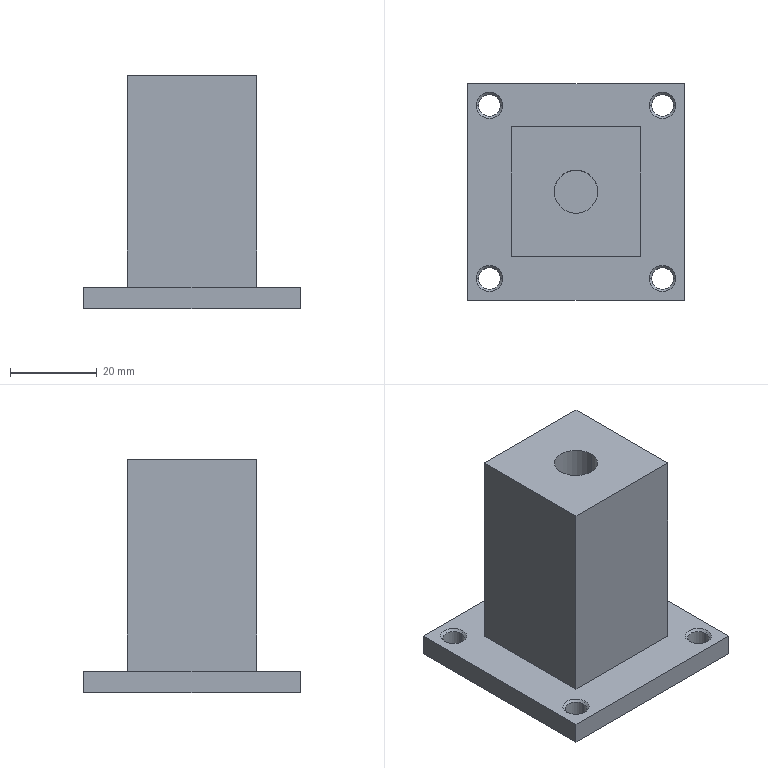Part | SolidWorks | features Cut 1, Extrusion 1, HoleWzd 1, ICE 1 | 1 solid | 30 faces | box 50 x 50 x 54 mm | volume 53135 mm3 | plane 12 | cylinder 10 | cone 8 | commonest cylinder face diameters 5 x8 10 x2
STEP:
#1=CARTESIAN_POINT('',(-55.,0.,15.));
#2=VERTEX_POINT('',#1);
#3=CARTESIAN_POINT('',(-45.,0.,15.));
#4=VERTEX_POINT('',#3);
#5=CARTESIAN_POINT('',(-50.,0.,15.));
#6=DIRECTION('',(0.,0.,1.));
#7=DIRECTION('',(1.,0.,0.));
#8=AXIS2_PLACEMENT_3D('',#5,#6,#7);
#9=CIRCLE('',#8,5.);
#10=EDGE_CURVE('',#2,#4,#9,.T.);
#11=ORIENTED_EDGE('',*,*,#10,.F.);
#12=CARTESIAN_POINT('',(-55.,0.,54.));
#13=VERTEX_POINT('',#12);
#14=CARTESIAN_POINT('',(-55.,0.,15.));
#15=DIRECTION('',(0.,0.,1.));
#16=VECTOR('',#15,1000.);
#17=LINE('',#14,#16);
#18=EDGE_CURVE('',#2,#13,#17,.T.);
#19=ORIENTED_EDGE('',*,*,#18,.T.);
#20=CARTESIAN_POINT('',(-45.,0.,54.));
#21=VERTEX_POINT('',#20);
#22=CARTESIAN_POINT('',(-50.,0.,54.));
#23=DIRECTION('',(0.,0.,1.));
#24=DIRECTION('',(1.,0.,0.));
#25=AXIS2_PLACEMENT_3D('',#22,#23,#24);
#26=CIRCLE('',#25,5.);
#27=EDGE_CURVE('',#13,#21,#26,.T.);
#28=ORIENTED_EDGE('',*,*,#27,.T.);
#29=CARTESIAN_POINT('',(-45.,0.,15.));
#30=DIRECTION('',(0.,0.,1.));
#31=VECTOR('',#30,1000.);
#32=LINE('',#29,#31);
#33=EDGE_CURVE('',#4,#21,#32,.T.);
#34=ORIENTED_EDGE('',*,*,#33,.F.);
#35=EDGE_LOOP('',(#11,#19,#28,#34));
#36=FACE_OUTER_BOUND('',#35,.T.);
#37=CARTESIAN_POINT('',(-50.,0.,15.));
#38=DIRECTION('',(0.,0.,1.));
#39=DIRECTION('',(1.,0.,0.));
#40=AXIS2_PLACEMENT_3D('',#37,#38,#39);
#41=CYLINDRICAL_SURFACE('',#40,5.);
#42=ADVANCED_FACE('',(#36),#41,.F.);
#43=CARTESIAN_POINT('',(-32.5,20.,4.475));
#44=VERTEX_POINT('',#43);
#45=CARTESIAN_POINT('',(-27.5,20.,4.475));
#46=VERTEX_POINT('',#45);
#47=CARTESIAN_POINT('',(-30.,20.,4.475));
#48=DIRECTION('',(0.,0.,1.));
#49=DIRECTION('',(1.,0.,0.));
#50=AXIS2_PLACEMENT_3D('',#47,#48,#49);
#51=CIRCLE('',#50,2.5);
#52=EDGE_CURVE('',#44,#46,#51,.T.);
#53=ORIENTED_EDGE('',*,*,#52,.F.);
#54=CARTESIAN_POINT('',(-33.025,20.,5.));
#55=VERTEX_POINT('',#54);
#56=CARTESIAN_POINT('',(-33.025,20.,5.));
#57=DIRECTION('',(-0.7071,0.,0.7071));
#58=VECTOR('',#57,1000.);
#59=LINE('',#56,#58);
#60=EDGE_CURVE('',#44,#55,#59,.T.);
#61=ORIENTED_EDGE('',*,*,#60,.T.);
#62=CARTESIAN_POINT('',(-26.975,20.,5.));
#63=VERTEX_POINT('',#62);
#64=CARTESIAN_POINT('',(-30.,20.,5.));
#65=DIRECTION('',(0.,0.,1.));
#66=DIRECTION('',(1.,0.,0.));
#67=AXIS2_PLACEMENT_3D('',#64,#65,#66);
#68=CIRCLE('',#67,3.025);
#69=EDGE_CURVE('',#55,#63,#68,.T.);
#70=ORIENTED_EDGE('',*,*,#69,.T.);
#71=CARTESIAN_POINT('',(-26.975,20.,5.));
#72=DIRECTION('',(0.7071,0.,0.7071));
#73=VECTOR('',#72,1000.);
#74=LINE('',#71,#73);
#75=EDGE_CURVE('',#46,#63,#74,.T.);
#76=ORIENTED_EDGE('',*,*,#75,.F.);
#77=EDGE_LOOP('',(#53,#61,#70,#76));
#78=FACE_OUTER_BOUND('',#77,.T.);
#79=CARTESIAN_POINT('',(-30.,20.,5.));
#80=DIRECTION('',(0.,0.,1.));
#81=DIRECTION('',(1.,0.,0.));
#82=AXIS2_PLACEMENT_3D('',#79,#80,#81);
#83=CONICAL_SURFACE('',#82,3.025,0.7854);
#84=ADVANCED_FACE('',(#78),#83,.F.);
#85=CARTESIAN_POINT('',(-27.5,20.,0.));
#86=VERTEX_POINT('',#85);
#87=CARTESIAN_POINT('',(-32.5,20.,0.));
#88=VERTEX_POINT('',#87);
#89=CARTESIAN_POINT('',(-30.,20.,0.));
#90=DIRECTION('',(0.,0.,-1.));
#91=DIRECTION('',(-1.,0.,0.));
#92=AXIS2_PLACEMENT_3D('',#89,#90,#91);
#93=CIRCLE('',#92,2.5);
#94=EDGE_CURVE('',#86,#88,#93,.T.);
#95=ORIENTED_EDGE('',*,*,#94,.T.);
#96=CARTESIAN_POINT('',(-32.5,20.,5.));
#97=DIRECTION('',(0.,0.,1.));
#98=VECTOR('',#97,1000.);
#99=LINE('',#96,#98);
#100=EDGE_CURVE('',#88,#44,#99,.T.);
#101=ORIENTED_EDGE('',*,*,#100,.T.);
#102=ORIENTED_EDGE('',*,*,#52,.T.);
#103=CARTESIAN_POINT('',(-27.5,20.,5.));
#104=DIRECTION('',(0.,0.,1.));
#105=VECTOR('',#104,1000.);
#106=LINE('',#103,#105);
#107=EDGE_CURVE('',#86,#46,#106,.T.);
#108=ORIENTED_EDGE('',*,*,#107,.F.);
#109=EDGE_LOOP('',(#95,#101,#102,#108));
#110=FACE_OUTER_BOUND('',#109,.T.);
#111=CARTESIAN_POINT('',(-30.,20.,5.));
#112=DIRECTION('',(0.,0.,1.));
#113=DIRECTION('',(1.,0.,0.));
#114=AXIS2_PLACEMENT_3D('',#111,#112,#113);
#115=CYLINDRICAL_SURFACE('',#114,2.5);
#116=ADVANCED_FACE('',(#110),#115,.F.);
#117=CARTESIAN_POINT('',(-72.5,20.,4.475));
#118=VERTEX_POINT('',#117);
#119=CARTESIAN_POINT('',(-67.5,20.,4.475));
#120=VERTEX_POINT('',#119);
#121=CARTESIAN_POINT('',(-70.,20.,4.475));
#122=DIRECTION('',(0.,0.,1.));
#123=DIRECTION('',(1.,0.,0.));
#124=AXIS2_PLACEMENT_3D('',#121,#122,#123);
#125=CIRCLE('',#124,2.5);
#126=EDGE_CURVE('',#118,#120,#125,.T.);
#127=ORIENTED_EDGE('',*,*,#126,.F.);
#128=CARTESIAN_POINT('',(-73.025,20.,5.));
#129=VERTEX_POINT('',#128);
#130=CARTESIAN_POINT('',(-73.025,20.,5.));
#131=DIRECTION('',(-0.7071,0.,0.7071));
#132=VECTOR('',#131,1000.);
#133=LINE('',#130,#132);
#134=EDGE_CURVE('',#118,#129,#133,.T.);
#135=ORIENTED_EDGE('',*,*,#134,.T.);
#136=CARTESIAN_POINT('',(-66.975,20.,5.));
#137=VERTEX_POINT('',#136);
#138=CARTESIAN_POINT('',(-70.,20.,5.));
#139=DIRECTION('',(0.,0.,1.));
#140=DIRECTION('',(1.,0.,0.));
#141=AXIS2_PLACEMENT_3D('',#138,#139,#140);
#142=CIRCLE('',#141,3.025);
#143=EDGE_CURVE('',#129,#137,#142,.T.);
#144=ORIENTED_EDGE('',*,*,#143,.T.);
#145=CARTESIAN_POINT('',(-66.975,20.,5.));
#146=DIRECTION('',(0.7071,0.,0.7071));
#147=VECTOR('',#146,1000.);
#148=LINE('',#145,#147);
#149=EDGE_CURVE('',#120,#137,#148,.T.);
#150=ORIENTED_EDGE('',*,*,#149,.F.);
#151=EDGE_LOOP('',(#127,#135,#144,#150));
#152=FACE_OUTER_BOUND('',#151,.T.);
#153=CARTESIAN_POINT('',(-70.,20.,5.));
#154=DIRECTION('',(0.,0.,1.));
#155=DIRECTION('',(1.,0.,0.));
#156=AXIS2_PLACEMENT_3D('',#153,#154,#155);
#157=CONICAL_SURFACE('',#156,3.025,0.7854);
#158=ADVANCED_FACE('',(#152),#157,.F.);
#159=CARTESIAN_POINT('',(-67.5,20.,0.));
#160=VERTEX_POINT('',#159);
#161=CARTESIAN_POINT('',(-72.5,20.,0.));
#162=VERTEX_POINT('',#161);
#163=CARTESIAN_POINT('',(-70.,20.,0.));
#164=DIRECTION('',(0.,0.,-1.));
#165=DIRECTION('',(-1.,0.,0.));
#166=AXIS2_PLACEMENT_3D('',#163,#164,#165);
#167=CIRCLE('',#166,2.5);
#168=EDGE_CURVE('',#160,#162,#167,.T.);
#169=ORIENTED_EDGE('',*,*,#168,.T.);
#170=CARTESIAN_POINT('',(-72.5,20.,5.));
#171=DIRECTION('',(0.,0.,1.));
#172=VECTOR('',#171,1000.);
#173=LINE('',#170,#172);
#174=EDGE_CURVE('',#162,#118,#173,.T.);
#175=ORIENTED_EDGE('',*,*,#174,.T.);
#176=ORIENTED_EDGE('',*,*,#126,.T.);
#177=CARTESIAN_POINT('',(-67.5,20.,5.));
#178=DIRECTION('',(0.,0.,1.));
#179=VECTOR('',#178,1000.);
#180=LINE('',#177,#179);
#181=EDGE_CURVE('',#160,#120,#180,.T.);
#182=ORIENTED_EDGE('',*,*,#181,.F.);
#183=EDGE_LOOP('',(#169,#175,#176,#182));
#184=FACE_OUTER_BOUND('',#183,.T.);
#185=CARTESIAN_POINT('',(-70.,20.,5.));
#186=DIRECTION('',(0.,0.,1.));
#187=DIRECTION('',(1.,0.,0.));
#188=AXIS2_PLACEMENT_3D('',#185,#186,#187);
#189=CYLINDRICAL_SURFACE('',#188,2.5);
#190=ADVANCED_FACE('',(#184),#189,.F.);
#191=CARTESIAN_POINT('',(-72.5,-20.,4.475));
#192=VERTEX_POINT('',#191);
#193=CARTESIAN_POINT('',(-67.5,-20.,4.475));
#194=VERTEX_POINT('',#193);
#195=CARTESIAN_POINT('',(-70.,-20.,4.475));
#196=DIRECTION('',(0.,0.,1.));
#197=DIRECTION('',(1.,0.,0.));
#198=AXIS2_PLACEMENT_3D('',#195,#196,#197);
#199=CIRCLE('',#198,2.5);
#200=EDGE_CURVE('',#192,#194,#199,.T.);
#201=ORIENTED_EDGE('',*,*,#200,.F.);
#202=CARTESIAN_POINT('',(-73.025,-20.,5.));
#203=VERTEX_POINT('',#202);
#204=CARTESIAN_POINT('',(-73.025,-20.,5.));
#205=DIRECTION('',(-0.7071,0.,0.7071));
#206=VECTOR('',#205,1000.);
#207=LINE('',#204,#206);
#208=EDGE_CURVE('',#192,#203,#207,.T.);
#209=ORIENTED_EDGE('',*,*,#208,.T.);
#210=CARTESIAN_POINT('',(-66.975,-20.,5.));
#211=VERTEX_POINT('',#210);
#212=CARTESIAN_POINT('',(-70.,-20.,5.));
#213=DIRECTION('',(0.,0.,1.));
#214=DIRECTION('',(1.,0.,0.));
#215=AXIS2_PLACEMENT_3D('',#212,#213,#214);
#216=CIRCLE('',#215,3.025);
#217=EDGE_CURVE('',#203,#211,#216,.T.);
#218=ORIENTED_EDGE('',*,*,#217,.T.);
#219=CARTESIAN_POINT('',(-66.975,-20.,5.));
#220=DIRECTION('',(0.7071,0.,0.7071));
#221=VECTOR('',#220,1000.);
#222=LINE('',#219,#221);
#223=EDGE_CURVE('',#194,#211,#222,.T.);
#224=ORIENTED_EDGE('',*,*,#223,.F.);
#225=EDGE_LOOP('',(#201,#209,#218,#224));
#226=FACE_OUTER_BOUND('',#225,.T.);
#227=CARTESIAN_POINT('',(-70.,-20.,5.));
#228=DIRECTION('',(0.,0.,1.));
#229=DIRECTION('',(1.,0.,0.));
#230=AXIS2_PLACEMENT_3D('',#227,#228,#229);
#231=CONICAL_SURFACE('',#230,3.025,0.7854);
#232=ADVANCED_FACE('',(#226),#231,.F.);
#233=CARTESIAN_POINT('',(-67.5,-20.,0.));
#234=VERTEX_POINT('',#233);
#235=CARTESIAN_POINT('',(-72.5,-20.,0.));
#236=VERTEX_POINT('',#235);
#237=CARTESIAN_POINT('',(-70.,-20.,0.));
#238=DIRECTION('',(0.,0.,-1.));
#239=DIRECTION('',(-1.,0.,0.));
#240=AXIS2_PLACEMENT_3D('',#237,#238,#239);
#241=CIRCLE('',#240,2.5);
#242=EDGE_CURVE('',#234,#236,#241,.T.);
#243=ORIENTED_EDGE('',*,*,#242,.T.);
#244=CARTESIAN_POINT('',(-72.5,-20.,5.));
#245=DIRECTION('',(0.,0.,1.));
#246=VECTOR('',#245,1000.);
#247=LINE('',#244,#246);
#248=EDGE_CURVE('',#236,#192,#247,.T.);
#249=ORIENTED_EDGE('',*,*,#248,.T.);
#250=ORIENTED_EDGE('',*,*,#200,.T.);
#251=CARTESIAN_POINT('',(-67.5,-20.,5.));
#252=DIRECTION('',(0.,0.,1.));
#253=VECTOR('',#252,1000.);
#254=LINE('',#251,#253);
#255=EDGE_CURVE('',#234,#194,#254,.T.);
#256=ORIENTED_EDGE('',*,*,#255,.F.);
#257=EDGE_LOOP('',(#243,#249,#250,#256));
#258=FACE_OUTER_BOUND('',#257,.T.);
#259=CARTESIAN_POINT('',(-70.,-20.,5.));
#260=DIRECTION('',(0.,0.,1.));
#261=DIRECTION('',(1.,0.,0.));
#262=AXIS2_PLACEMENT_3D('',#259,#260,#261);
#263=CYLINDRICAL_SURFACE('',#262,2.5);
#264=ADVANCED_FACE('',(#258),#263,.F.);
#265=CARTESIAN_POINT('',(-32.5,-20.,4.475));
#266=VERTEX_POINT('',#265);
#267=CARTESIAN_POINT('',(-27.5,-20.,4.475));
#268=VERTEX_POINT('',#267);
#269=CARTESIAN_POINT('',(-30.,-20.,4.475));
#270=DIRECTION('',(0.,0.,1.));
#271=DIRECTION('',(1.,0.,0.));
#272=AXIS2_PLACEMENT_3D('',#269,#270,#271);
#273=CIRCLE('',#272,2.5);
#274=EDGE_CURVE('',#266,#268,#273,.T.);
#275=ORIENTED_EDGE('',*,*,#274,.F.);
#276=CARTESIAN_POINT('',(-33.025,-20.,5.));
#277=VERTEX_POINT('',#276);
#278=CARTESIAN_POINT('',(-33.025,-20.,5.));
#279=DIRECTION('',(-0.7071,0.,0.7071));
#280=VECTOR('',#279,1000.);
#281=LINE('',#278,#280);
#282=EDGE_CURVE('',#266,#277,#281,.T.);
#283=ORIENTED_EDGE('',*,*,#282,.T.);
#284=CARTESIAN_POINT('',(-26.975,-20.,5.));
#285=VERTEX_POINT('',#284);
#286=CARTESIAN_POINT('',(-30.,-20.,5.));
#287=DIRECTION('',(0.,0.,1.));
#288=DIRECTION('',(1.,0.,0.));
#289=AXIS2_PLACEMENT_3D('',#286,#287,#288);
#290=CIRCLE('',#289,3.025);
#291=EDGE_CURVE('',#277,#285,#290,.T.);
#292=ORIENTED_EDGE('',*,*,#291,.T.);
#293=CARTESIAN_POINT('',(-26.975,-20.,5.));
#294=DIRECTION('',(0.7071,0.,0.7071));
#295=VECTOR('',#294,1000.);
#296=LINE('',#293,#295);
#297=EDGE_CURVE('',#268,#285,#296,.T.);
#298=ORIENTED_EDGE('',*,*,#297,.F.);
#299=EDGE_LOOP('',(#275,#283,#292,#298));
#300=FACE_OUTER_BOUND('',#299,.T.);
#301=CARTESIAN_POINT('',(-30.,-20.,5.));
#302=DIRECTION('',(0.,0.,1.));
#303=DIRECTION('',(1.,0.,0.));
#304=AXIS2_PLACEMENT_3D('',#301,#302,#303);
#305=CONICAL_SURFACE('',#304,3.025,0.7854);
#306=ADVANCED_FACE('',(#300),#305,.F.);
#307=CARTESIAN_POINT('',(-27.5,-20.,0.));
#308=VERTEX_POINT('',#307);
#309=CARTESIAN_POINT('',(-32.5,-20.,0.));
#310=VERTEX_POINT('',#309);
#311=CARTESIAN_POINT('',(-30.,-20.,0.));
#312=DIRECTION('',(0.,0.,-1.));
#313=DIRECTION('',(-1.,0.,0.));
#314=AXIS2_PLACEMENT_3D('',#311,#312,#313);
#315=CIRCLE('',#314,2.5);
#316=EDGE_CURVE('',#308,#310,#315,.T.);
#317=ORIENTED_EDGE('',*,*,#316,.T.);
#318=CARTESIAN_POINT('',(-32.5,-20.,5.));
#319=DIRECTION('',(0.,0.,1.));
#320=VECTOR('',#319,1000.);
#321=LINE('',#318,#320);
#322=EDGE_CURVE('',#310,#266,#321,.T.);
#323=ORIENTED_EDGE('',*,*,#322,.T.);
#324=ORIENTED_EDGE('',*,*,#274,.T.);
#325=CARTESIAN_POINT('',(-27.5,-20.,5.));
#326=DIRECTION('',(0.,0.,1.));
#327=VECTOR('',#326,1000.);
#328=LINE('',#325,#327);
#329=EDGE_CURVE('',#308,#268,#328,.T.);
#330=ORIENTED_EDGE('',*,*,#329,.F.);
#331=EDGE_LOOP('',(#317,#323,#324,#330));
#332=FACE_OUTER_BOUND('',#331,.T.);
#333=CARTESIAN_POINT('',(-30.,-20.,5.));
#334=DIRECTION('',(0.,0.,1.));
#335=DIRECTION('',(1.,0.,0.));
#336=AXIS2_PLACEMENT_3D('',#333,#334,#335);
#337=CYLINDRICAL_SURFACE('',#336,2.5);
#338=ADVANCED_FACE('',(#332),#337,.F.);
#339=CARTESIAN_POINT('',(-65.,15.,54.));
#340=VERTEX_POINT('',#339);
#341=CARTESIAN_POINT('',(-65.,15.,5.));
#342=VERTEX_POINT('',#341);
#343=CARTESIAN_POINT('',(-65.,15.,54.));
#344=DIRECTION('',(0.,0.,-1.));
#345=VECTOR('',#344,1000.);
#346=LINE('',#343,#345);
#347=EDGE_CURVE('',#340,#342,#346,.T.);
#348=ORIENTED_EDGE('',*,*,#347,.T.);
#349=CARTESIAN_POINT('',(-65.,-15.,5.));
#350=VERTEX_POINT('',#349);
#351=CARTESIAN_POINT('',(-65.,15.,5.));
#352=DIRECTION('',(0.,-1.,0.));
#353=VECTOR('',#352,1000.);
#354=LINE('',#351,#353);
#355=EDGE_CURVE('',#342,#350,#354,.T.);
#356=ORIENTED_EDGE('',*,*,#355,.T.);
#357=CARTESIAN_POINT('',(-65.,-15.,54.));
#358=VERTEX_POINT('',#357);
#359=CARTESIAN_POINT('',(-65.,-15.,54.));
#360=DIRECTION('',(0.,0.,-1.));
#361=VECTOR('',#360,1000.);
#362=LINE('',#359,#361);
#363=EDGE_CURVE('',#358,#350,#362,.T.);
#364=ORIENTED_EDGE('',*,*,#363,.F.);
#365=CARTESIAN_POINT('',(-65.,15.,54.));
#366=DIRECTION('',(0.,-1.,0.));
#367=VECTOR('',#366,1000.);
#368=LINE('',#365,#367);
#369=EDGE_CURVE('',#340,#358,#368,.T.);
#370=ORIENTED_EDGE('',*,*,#369,.F.);
#371=EDGE_LOOP('',(#348,#356,#364,#370));
#372=FACE_OUTER_BOUND('',#371,.T.);
#373=CARTESIAN_POINT('',(-65.,15.,54.));
#374=DIRECTION('',(1.,0.,0.));
#375=DIRECTION('',(0.,0.,-1.));
#376=AXIS2_PLACEMENT_3D('',#373,#374,#375);
#377=PLANE('',#376);
#378=ADVANCED_FACE('',(#372),#377,.F.);
#379=ORIENTED_EDGE('',*,*,#363,.T.);
#380=CARTESIAN_POINT('',(-35.,-15.,5.));
#381=VERTEX_POINT('',#380);
#382=CARTESIAN_POINT('',(-35.,-15.,5.));
#383=DIRECTION('',(1.,0.,0.));
#384=VECTOR('',#383,1000.);
#385=LINE('',#382,#384);
#386=EDGE_CURVE('',#350,#381,#385,.T.);
#387=ORIENTED_EDGE('',*,*,#386,.T.);
#388=CARTESIAN_POINT('',(-35.,-15.,54.));
#389=VERTEX_POINT('',#388);
#390=CARTESIAN_POINT('',(-35.,-15.,54.));
#391=DIRECTION('',(0.,0.,-1.));
#392=VECTOR('',#391,1000.);
#393=LINE('',#390,#392);
#394=EDGE_CURVE('',#389,#381,#393,.T.);
#395=ORIENTED_EDGE('',*,*,#394,.F.);
#396=CARTESIAN_POINT('',(-35.,-15.,54.));
#397=DIRECTION('',(1.,0.,0.));
#398=VECTOR('',#397,1000.);
#399=LINE('',#396,#398);
#400=EDGE_CURVE('',#358,#389,#399,.T.);
#401=ORIENTED_EDGE('',*,*,#400,.F.);
#402=EDGE_LOOP('',(#379,#387,#395,#401));
#403=FACE_OUTER_BOUND('',#402,.T.);
#404=CARTESIAN_POINT('',(-35.,-15.,54.));
#405=DIRECTION('',(0.,1.,0.));
#406=DIRECTION('',(-1.,0.,0.));
#407=AXIS2_PLACEMENT_3D('',#404,#405,#406);
#408=PLANE('',#407);
#409=ADVANCED_FACE('',(#403),#408,.F.);
#410=ORIENTED_EDGE('',*,*,#394,.T.);
#411=CARTESIAN_POINT('',(-35.,15.,5.));
#412=VERTEX_POINT('',#411);
#413=CARTESIAN_POINT('',(-35.,15.,5.));
#414=DIRECTION('',(0.,1.,0.));
#415=VECTOR('',#414,1000.);
#416=LINE('',#413,#415);
#417=EDGE_CURVE('',#381,#412,#416,.T.);
#418=ORIENTED_EDGE('',*,*,#417,.T.);
#419=CARTESIAN_POINT('',(-35.,15.,54.));
#420=VERTEX_POINT('',#419);
#421=CARTESIAN_POINT('',(-35.,15.,54.));
#422=DIRECTION('',(0.,0.,-1.));
#423=VECTOR('',#422,1000.);
#424=LINE('',#421,#423);
#425=EDGE_CURVE('',#420,#412,#424,.T.);
#426=ORIENTED_EDGE('',*,*,#425,.F.);
#427=CARTESIAN_POINT('',(-35.,15.,54.));
#428=DIRECTION('',(0.,1.,0.));
#429=VECTOR('',#428,1000.);
#430=LINE('',#427,#429);
#431=EDGE_CURVE('',#389,#420,#430,.T.);
#432=ORIENTED_EDGE('',*,*,#431,.F.);
#433=EDGE_LOOP('',(#410,#418,#426,#432));
#434=FACE_OUTER_BOUND('',#433,.T.);
#435=CARTESIAN_POINT('',(-35.,15.,54.));
#436=DIRECTION('',(-1.,0.,0.));
#437=DIRECTION('',(0.,-1.,0.));
#438=AXIS2_PLACEMENT_3D('',#435,#436,#437);
#439=PLANE('',#438);
#440=ADVANCED_FACE('',(#434),#439,.F.);
#441=ORIENTED_EDGE('',*,*,#425,.T.);
#442=CARTESIAN_POINT('',(-35.,15.,5.));
#443=DIRECTION('',(-1.,0.,0.));
#444=VECTOR('',#443,1000.);
#445=LINE('',#442,#444);
#446=EDGE_CURVE('',#412,#342,#445,.T.);
#447=ORIENTED_EDGE('',*,*,#446,.T.);
#448=ORIENTED_EDGE('',*,*,#347,.F.);
#449=CARTESIAN_POINT('',(-35.,15.,54.));
#450=DIRECTION('',(-1.,0.,0.));
#451=VECTOR('',#450,1000.);
#452=LINE('',#449,#451);
#453=EDGE_CURVE('',#420,#340,#452,.T.);
#454=ORIENTED_EDGE('',*,*,#453,.F.);
#455=EDGE_LOOP('',(#441,#447,#448,#454));
#456=FACE_OUTER_BOUND('',#455,.T.);
#457=CARTESIAN_POINT('',(-35.,15.,54.));
#458=DIRECTION('',(0.,-1.,0.));
#459=DIRECTION('',(1.,0.,0.));
#460=AXIS2_PLACEMENT_3D('',#457,#458,#459);
#461=PLANE('',#460);
#462=ADVANCED_FACE('',(#456),#461,.F.);
#463=CARTESIAN_POINT('',(-50.,0.,54.));
#464=DIRECTION('',(0.,0.,1.));
#465=DIRECTION('',(1.,0.,0.));
#466=AXIS2_PLACEMENT_3D('',#463,#464,#465);
#467=CIRCLE('',#466,5.);
#468=EDGE_CURVE('',#21,#13,#467,.T.);
#469=ORIENTED_EDGE('',*,*,#468,.F.);
#470=ORIENTED_EDGE('',*,*,#27,.F.);
#471=EDGE_LOOP('',(#469,#470));
#472=FACE_BOUND('',#471,.T.);
#473=ORIENTED_EDGE('',*,*,#369,.T.);
#474=ORIENTED_EDGE('',*,*,#400,.T.);
#475=ORIENTED_EDGE('',*,*,#431,.T.);
#476=ORIENTED_EDGE('',*,*,#453,.T.);
#477=EDGE_LOOP('',(#473,#474,#475,#476));
#478=FACE_OUTER_BOUND('',#477,.T.);
#479=CARTESIAN_POINT('',(0.,0.,54.));
#480=DIRECTION('',(0.,0.,-1.));
#481=DIRECTION('',(-1.,0.,0.));
#482=AXIS2_PLACEMENT_3D('',#479,#480,#481);
#483=PLANE('',#482);
#484=ADVANCED_FACE('',(#472,#478),#483,.F.);
#485=CARTESIAN_POINT('',(-30.,20.,5.));
#486=DIRECTION('',(0.,0.,1.));
#487=DIRECTION('',(1.,0.,0.));
#488=AXIS2_PLACEMENT_3D('',#485,#486,#487);
#489=CIRCLE('',#488,3.025);
#490=EDGE_CURVE('',#63,#55,#489,.T.);
#491=ORIENTED_EDGE('',*,*,#490,.F.);
#492=ORIENTED_EDGE('',*,*,#69,.F.);
#493=EDGE_LOOP('',(#491,#492));
#494=FACE_BOUND('',#493,.T.);
#495=CARTESIAN_POINT('',(-70.,20.,5.));
#496=DIRECTION('',(0.,0.,1.));
#497=DIRECTION('',(1.,0.,0.));
#498=AXIS2_PLACEMENT_3D('',#495,#496,#497);
#499=CIRCLE('',#498,3.025);
#500=EDGE_CURVE('',#137,#129,#499,.T.);
#501=ORIENTED_EDGE('',*,*,#500,.F.);
#502=ORIENTED_EDGE('',*,*,#143,.F.);
#503=EDGE_LOOP('',(#501,#502));
#504=FACE_BOUND('',#503,.T.);
#505=CARTESIAN_POINT('',(-70.,-20.,5.));
#506=DIRECTION('',(0.,0.,1.));
#507=DIRECTION('',(1.,0.,0.));
#508=AXIS2_PLACEMENT_3D('',#505,#506,#507);
#509=CIRCLE('',#508,3.025);
#510=EDGE_CURVE('',#211,#203,#509,.T.);
#511=ORIENTED_EDGE('',*,*,#510,.F.);
#512=ORIENTED_EDGE('',*,*,#217,.F.);
#513=EDGE_LOOP('',(#511,#512));
#514=FACE_BOUND('',#513,.T.);
#515=CARTESIAN_POINT('',(-30.,-20.,5.));
#516=DIRECTION('',(0.,0.,1.));
#517=DIRECTION('',(1.,0.,0.));
#518=AXIS2_PLACEMENT_3D('',#515,#516,#517);
#519=CIRCLE('',#518,3.025);
#520=EDGE_CURVE('',#285,#277,#519,.T.);
#521=ORIENTED_EDGE('',*,*,#520,.F.);
#522=ORIENTED_EDGE('',*,*,#291,.F.);
#523=EDGE_LOOP('',(#521,#522));
#524=FACE_BOUND('',#523,.T.);
#525=CARTESIAN_POINT('',(-25.,25.,5.));
#526=VERTEX_POINT('',#525);
#527=CARTESIAN_POINT('',(-75.,25.,5.));
#528=VERTEX_POINT('',#527);
#529=CARTESIAN_POINT('',(-25.,25.,5.));
#530=DIRECTION('',(-1.,0.,0.));
#531=VECTOR('',#530,1000.);
#532=LINE('',#529,#531);
#533=EDGE_CURVE('',#526,#528,#532,.T.);
#534=ORIENTED_EDGE('',*,*,#533,.T.);
#535=CARTESIAN_POINT('',(-75.,-25.,5.));
#536=VERTEX_POINT('',#535);
#537=CARTESIAN_POINT('',(-75.,25.,5.));
#538=DIRECTION('',(0.,-1.,0.));
#539=VECTOR('',#538,1000.);
#540=LINE('',#537,#539);
#541=EDGE_CURVE('',#528,#536,#540,.T.);
#542=ORIENTED_EDGE('',*,*,#541,.T.);
#543=CARTESIAN_POINT('',(-25.,-25.,5.));
#544=VERTEX_POINT('',#543);
#545=CARTESIAN_POINT('',(-75.,-25.,5.));
#546=DIRECTION('',(1.,0.,0.));
#547=VECTOR('',#546,1000.);
#548=LINE('',#545,#547);
#549=EDGE_CURVE('',#536,#544,#548,.T.);
#550=ORIENTED_EDGE('',*,*,#549,.T.);
#551=CARTESIAN_POINT('',(-25.,-25.,5.));
#552=DIRECTION('',(0.,1.,0.));
#553=VECTOR('',#552,1000.);
#554=LINE('',#551,#553);
#555=EDGE_CURVE('',#544,#526,#554,.T.);
#556=ORIENTED_EDGE('',*,*,#555,.T.);
#557=EDGE_LOOP('',(#534,#542,#550,#556));
#558=FACE_OUTER_BOUND('',#557,.T.);
#559=ORIENTED_EDGE('',*,*,#355,.F.);
#560=ORIENTED_EDGE('',*,*,#446,.F.);
#561=ORIENTED_EDGE('',*,*,#417,.F.);
#562=ORIENTED_EDGE('',*,*,#386,.F.);
#563=EDGE_LOOP('',(#559,#560,#561,#562));
#564=FACE_BOUND('',#563,.T.);
#565=CARTESIAN_POINT('',(0.,0.,5.));
#566=DIRECTION('',(0.,0.,1.));
#567=DIRECTION('',(1.,0.,0.));
#568=AXIS2_PLACEMENT_3D('',#565,#566,#567);
#569=PLANE('',#568);
#570=ADVANCED_FACE('',(#494,#504,#514,#524,#558,#564),#569,.T.);
#571=CARTESIAN_POINT('',(-25.,25.,0.));
#572=VERTEX_POINT('',#571);
#573=CARTESIAN_POINT('',(-75.,25.,0.));
#574=VERTEX_POINT('',#573);
#575=CARTESIAN_POINT('',(-25.,25.,0.));
#576=DIRECTION('',(-1.,0.,0.));
#577=VECTOR('',#576,1000.);
#578=LINE('',#575,#577);
#579=EDGE_CURVE('',#572,#574,#578,.T.);
#580=ORIENTED_EDGE('',*,*,#579,.T.);
#581=CARTESIAN_POINT('',(-75.,25.,5.));
#582=DIRECTION('',(0.,0.,-1.));
#583=VECTOR('',#582,1000.);
#584=LINE('',#581,#583);
#585=EDGE_CURVE('',#528,#574,#584,.T.);
#586=ORIENTED_EDGE('',*,*,#585,.F.);
#587=ORIENTED_EDGE('',*,*,#533,.F.);
#588=CARTESIAN_POINT('',(-25.,25.,5.));
#589=DIRECTION('',(0.,0.,-1.));
#590=VECTOR('',#589,1000.);
#591=LINE('',#588,#590);
#592=EDGE_CURVE('',#526,#572,#591,.T.);
#593=ORIENTED_EDGE('',*,*,#592,.T.);
#594=EDGE_LOOP('',(#580,#586,#587,#593));
#595=FACE_OUTER_BOUND('',#594,.T.);
#596=CARTESIAN_POINT('',(-25.,25.,5.));
#597=DIRECTION('',(0.,-1.,0.));
#598=DIRECTION('',(1.,0.,0.));
#599=AXIS2_PLACEMENT_3D('',#596,#597,#598);
#600=PLANE('',#599);
#601=ADVANCED_FACE('',(#595),#600,.F.);
#602=CARTESIAN_POINT('',(-75.,-25.,0.));
#603=VERTEX_POINT('',#602);
#604=CARTESIAN_POINT('',(-75.,25.,0.));
#605=DIRECTION('',(0.,-1.,0.));
#606=VECTOR('',#605,1000.);
#607=LINE('',#604,#606);
#608=EDGE_CURVE('',#574,#603,#607,.T.);
#609=ORIENTED_EDGE('',*,*,#608,.T.);
#610=CARTESIAN_POINT('',(-75.,-25.,5.));
#611=DIRECTION('',(0.,0.,-1.));
#612=VECTOR('',#611,1000.);
#613=LINE('',#610,#612);
#614=EDGE_CURVE('',#536,#603,#613,.T.);
#615=ORIENTED_EDGE('',*,*,#614,.F.);
#616=ORIENTED_EDGE('',*,*,#541,.F.);
#617=ORIENTED_EDGE('',*,*,#585,.T.);
#618=EDGE_LOOP('',(#609,#615,#616,#617));
#619=FACE_OUTER_BOUND('',#618,.T.);
#620=CARTESIAN_POINT('',(-75.,25.,5.));
#621=DIRECTION('',(1.,0.,0.));
#622=DIRECTION('',(0.,0.,-1.));
#623=AXIS2_PLACEMENT_3D('',#620,#621,#622);
#624=PLANE('',#623);
#625=ADVANCED_FACE('',(#619),#624,.F.);
#626=CARTESIAN_POINT('',(-25.,-25.,0.));
#627=VERTEX_POINT('',#626);
#628=CARTESIAN_POINT('',(-75.,-25.,0.));
#629=DIRECTION('',(1.,0.,0.));
#630=VECTOR('',#629,1000.);
#631=LINE('',#628,#630);
#632=EDGE_CURVE('',#603,#627,#631,.T.);
#633=ORIENTED_EDGE('',*,*,#632,.T.);
#634=CARTESIAN_POINT('',(-25.,-25.,5.));
#635=DIRECTION('',(0.,0.,-1.));
#636=VECTOR('',#635,1000.);
#637=LINE('',#634,#636);
#638=EDGE_CURVE('',#544,#627,#637,.T.);
#639=ORIENTED_EDGE('',*,*,#638,.F.);
#640=ORIENTED_EDGE('',*,*,#549,.F.);
#641=ORIENTED_EDGE('',*,*,#614,.T.);
#642=EDGE_LOOP('',(#633,#639,#640,#641));
#643=FACE_OUTER_BOUND('',#642,.T.);
#644=CARTESIAN_POINT('',(-75.,-25.,5.));
#645=DIRECTION('',(0.,1.,0.));
#646=DIRECTION('',(-1.,0.,0.));
#647=AXIS2_PLACEMENT_3D('',#644,#645,#646);
#648=PLANE('',#647);
#649=ADVANCED_FACE('',(#643),#648,.F.);
#650=CARTESIAN_POINT('',(-25.,-25.,0.));
#651=DIRECTION('',(0.,1.,0.));
#652=VECTOR('',#651,1000.);
#653=LINE('',#650,#652);
#654=EDGE_CURVE('',#627,#572,#653,.T.);
#655=ORIENTED_EDGE('',*,*,#654,.T.);
#656=ORIENTED_EDGE('',*,*,#592,.F.);
#657=ORIENTED_EDGE('',*,*,#555,.F.);
#658=ORIENTED_EDGE('',*,*,#638,.T.);
#659=EDGE_LOOP('',(#655,#656,#657,#658));
#660=FACE_OUTER_BOUND('',#659,.T.);
#661=CARTESIAN_POINT('',(-25.,-25.,5.));
#662=DIRECTION('',(-1.,0.,0.));
#663=DIRECTION('',(0.,-1.,0.));
#664=AXIS2_PLACEMENT_3D('',#661,#662,#663);
#665=PLANE('',#664);
#666=ADVANCED_FACE('',(#660),#665,.F.);
#667=ORIENTED_EDGE('',*,*,#94,.F.);
#668=CARTESIAN_POINT('',(-30.,20.,0.));
#669=DIRECTION('',(0.,0.,-1.));
#670=DIRECTION('',(-1.,0.,0.));
#671=AXIS2_PLACEMENT_3D('',#668,#669,#670);
#672=CIRCLE('',#671,2.5);
#673=EDGE_CURVE('',#88,#86,#672,.T.);
#674=ORIENTED_EDGE('',*,*,#673,.F.);
#675=EDGE_LOOP('',(#667,#674));
#676=FACE_BOUND('',#675,.T.);
#677=ORIENTED_EDGE('',*,*,#168,.F.);
#678=CARTESIAN_POINT('',(-70.,20.,0.));
#679=DIRECTION('',(0.,0.,-1.));
#680=DIRECTION('',(-1.,0.,0.));
#681=AXIS2_PLACEMENT_3D('',#678,#679,#680);
#682=CIRCLE('',#681,2.5);
#683=EDGE_CURVE('',#162,#160,#682,.T.);
#684=ORIENTED_EDGE('',*,*,#683,.F.);
#685=EDGE_LOOP('',(#677,#684));
#686=FACE_BOUND('',#685,.T.);
#687=ORIENTED_EDGE('',*,*,#242,.F.);
#688=CARTESIAN_POINT('',(-70.,-20.,0.));
#689=DIRECTION('',(0.,0.,-1.));
#690=DIRECTION('',(-1.,0.,0.));
#691=AXIS2_PLACEMENT_3D('',#688,#689,#690);
#692=CIRCLE('',#691,2.5);
#693=EDGE_CURVE('',#236,#234,#692,.T.);
#694=ORIENTED_EDGE('',*,*,#693,.F.);
#695=EDGE_LOOP('',(#687,#694));
#696=FACE_BOUND('',#695,.T.);
#697=ORIENTED_EDGE('',*,*,#316,.F.);
#698=CARTESIAN_POINT('',(-30.,-20.,0.));
#699=DIRECTION('',(0.,0.,-1.));
#700=DIRECTION('',(-1.,0.,0.));
#701=AXIS2_PLACEMENT_3D('',#698,#699,#700);
#702=CIRCLE('',#701,2.5);
#703=EDGE_CURVE('',#310,#308,#702,.T.);
#704=ORIENTED_EDGE('',*,*,#703,.F.);
#705=EDGE_LOOP('',(#697,#704));
#706=FACE_BOUND('',#705,.T.);
#707=ORIENTED_EDGE('',*,*,#579,.F.);
#708=ORIENTED_EDGE('',*,*,#654,.F.);
#709=ORIENTED_EDGE('',*,*,#632,.F.);
#710=ORIENTED_EDGE('',*,*,#608,.F.);
#711=EDGE_LOOP('',(#707,#708,#709,#710));
#712=FACE_OUTER_BOUND('',#711,.T.);
#713=CARTESIAN_POINT('',(0.,0.,0.));
#714=DIRECTION('',(0.,0.,-1.));
#715=DIRECTION('',(-1.,0.,0.));
#716=AXIS2_PLACEMENT_3D('',#713,#714,#715);
#717=PLANE('',#716);
#718=ADVANCED_FACE('',(#676,#686,#696,#706,#712),#717,.T.);
#719=ORIENTED_EDGE('',*,*,#322,.F.);
#720=ORIENTED_EDGE('',*,*,#703,.T.);
#721=ORIENTED_EDGE('',*,*,#329,.T.);
#722=CARTESIAN_POINT('',(-30.,-20.,4.475));
#723=DIRECTION('',(0.,0.,1.));
#724=DIRECTION('',(1.,0.,0.));
#725=AXIS2_PLACEMENT_3D('',#722,#723,#724);
#726=CIRCLE('',#725,2.5);
#727=EDGE_CURVE('',#268,#266,#726,.T.);
#728=ORIENTED_EDGE('',*,*,#727,.T.);
#729=EDGE_LOOP('',(#719,#720,#721,#728));
#730=FACE_OUTER_BOUND('',#729,.T.);
#731=CARTESIAN_POINT('',(-30.,-20.,5.));
#732=DIRECTION('',(0.,0.,1.));
#733=DIRECTION('',(1.,0.,0.));
#734=AXIS2_PLACEMENT_3D('',#731,#732,#733);
#735=CYLINDRICAL_SURFACE('',#734,2.5);
#736=ADVANCED_FACE('',(#730),#735,.F.);
#737=ORIENTED_EDGE('',*,*,#282,.F.);
#738=ORIENTED_EDGE('',*,*,#727,.F.);
#739=ORIENTED_EDGE('',*,*,#297,.T.);
#740=ORIENTED_EDGE('',*,*,#520,.T.);
#741=EDGE_LOOP('',(#737,#738,#739,#740));
#742=FACE_OUTER_BOUND('',#741,.T.);
#743=CARTESIAN_POINT('',(-30.,-20.,5.));
#744=DIRECTION('',(0.,0.,1.));
#745=DIRECTION('',(1.,0.,0.));
#746=AXIS2_PLACEMENT_3D('',#743,#744,#745);
#747=CONICAL_SURFACE('',#746,3.025,0.7854);
#748=ADVANCED_FACE('',(#742),#747,.F.);
#749=ORIENTED_EDGE('',*,*,#248,.F.);
#750=ORIENTED_EDGE('',*,*,#693,.T.);
#751=ORIENTED_EDGE('',*,*,#255,.T.);
#752=CARTESIAN_POINT('',(-70.,-20.,4.475));
#753=DIRECTION('',(0.,0.,1.));
#754=DIRECTION('',(1.,0.,0.));
#755=AXIS2_PLACEMENT_3D('',#752,#753,#754);
#756=CIRCLE('',#755,2.5);
#757=EDGE_CURVE('',#194,#192,#756,.T.);
#758=ORIENTED_EDGE('',*,*,#757,.T.);
#759=EDGE_LOOP('',(#749,#750,#751,#758));
#760=FACE_OUTER_BOUND('',#759,.T.);
#761=CARTESIAN_POINT('',(-70.,-20.,5.));
#762=DIRECTION('',(0.,0.,1.));
#763=DIRECTION('',(1.,0.,0.));
#764=AXIS2_PLACEMENT_3D('',#761,#762,#763);
#765=CYLINDRICAL_SURFACE('',#764,2.5);
#766=ADVANCED_FACE('',(#760),#765,.F.);
#767=ORIENTED_EDGE('',*,*,#208,.F.);
#768=ORIENTED_EDGE('',*,*,#757,.F.);
#769=ORIENTED_EDGE('',*,*,#223,.T.);
#770=ORIENTED_EDGE('',*,*,#510,.T.);
#771=EDGE_LOOP('',(#767,#768,#769,#770));
#772=FACE_OUTER_BOUND('',#771,.T.);
#773=CARTESIAN_POINT('',(-70.,-20.,5.));
#774=DIRECTION('',(0.,0.,1.));
#775=DIRECTION('',(1.,0.,0.));
#776=AXIS2_PLACEMENT_3D('',#773,#774,#775);
#777=CONICAL_SURFACE('',#776,3.025,0.7854);
#778=ADVANCED_FACE('',(#772),#777,.F.);
#779=ORIENTED_EDGE('',*,*,#174,.F.);
#780=ORIENTED_EDGE('',*,*,#683,.T.);
#781=ORIENTED_EDGE('',*,*,#181,.T.);
#782=CARTESIAN_POINT('',(-70.,20.,4.475));
#783=DIRECTION('',(0.,0.,1.));
#784=DIRECTION('',(1.,0.,0.));
#785=AXIS2_PLACEMENT_3D('',#782,#783,#784);
#786=CIRCLE('',#785,2.5);
#787=EDGE_CURVE('',#120,#118,#786,.T.);
#788=ORIENTED_EDGE('',*,*,#787,.T.);
#789=EDGE_LOOP('',(#779,#780,#781,#788));
#790=FACE_OUTER_BOUND('',#789,.T.);
#791=CARTESIAN_POINT('',(-70.,20.,5.));
#792=DIRECTION('',(0.,0.,1.));
#793=DIRECTION('',(1.,0.,0.));
#794=AXIS2_PLACEMENT_3D('',#791,#792,#793);
#795=CYLINDRICAL_SURFACE('',#794,2.5);
#796=ADVANCED_FACE('',(#790),#795,.F.);
#797=ORIENTED_EDGE('',*,*,#134,.F.);
#798=ORIENTED_EDGE('',*,*,#787,.F.);
#799=ORIENTED_EDGE('',*,*,#149,.T.);
#800=ORIENTED_EDGE('',*,*,#500,.T.);
#801=EDGE_LOOP('',(#797,#798,#799,#800));
#802=FACE_OUTER_BOUND('',#801,.T.);
#803=CARTESIAN_POINT('',(-70.,20.,5.));
#804=DIRECTION('',(0.,0.,1.));
#805=DIRECTION('',(1.,0.,0.));
#806=AXIS2_PLACEMENT_3D('',#803,#804,#805);
#807=CONICAL_SURFACE('',#806,3.025,0.7854);
#808=ADVANCED_FACE('',(#802),#807,.F.);
#809=ORIENTED_EDGE('',*,*,#100,.F.);
#810=ORIENTED_EDGE('',*,*,#673,.T.);
#811=ORIENTED_EDGE('',*,*,#107,.T.);
#812=CARTESIAN_POINT('',(-30.,20.,4.475));
#813=DIRECTION('',(0.,0.,1.));
#814=DIRECTION('',(1.,0.,0.));
#815=AXIS2_PLACEMENT_3D('',#812,#813,#814);
#816=CIRCLE('',#815,2.5);
#817=EDGE_CURVE('',#46,#44,#816,.T.);
#818=ORIENTED_EDGE('',*,*,#817,.T.);
#819=EDGE_LOOP('',(#809,#810,#811,#818));
#820=FACE_OUTER_BOUND('',#819,.T.);
#821=CARTESIAN_POINT('',(-30.,20.,5.));
#822=DIRECTION('',(0.,0.,1.));
#823=DIRECTION('',(1.,0.,0.));
#824=AXIS2_PLACEMENT_3D('',#821,#822,#823);
#825=CYLINDRICAL_SURFACE('',#824,2.5);
#826=ADVANCED_FACE('',(#820),#825,.F.);
#827=ORIENTED_EDGE('',*,*,#60,.F.);
#828=ORIENTED_EDGE('',*,*,#817,.F.);
#829=ORIENTED_EDGE('',*,*,#75,.T.);
#830=ORIENTED_EDGE('',*,*,#490,.T.);
#831=EDGE_LOOP('',(#827,#828,#829,#830));
#832=FACE_OUTER_BOUND('',#831,.T.);
#833=CARTESIAN_POINT('',(-30.,20.,5.));
#834=DIRECTION('',(0.,0.,1.));
#835=DIRECTION('',(1.,0.,0.));
#836=AXIS2_PLACEMENT_3D('',#833,#834,#835);
#837=CONICAL_SURFACE('',#836,3.025,0.7854);
#838=ADVANCED_FACE('',(#832),#837,.F.);
#839=ORIENTED_EDGE('',*,*,#18,.F.);
#840=CARTESIAN_POINT('',(-50.,0.,15.));
#841=DIRECTION('',(0.,0.,1.));
#842=DIRECTION('',(1.,0.,0.));
#843=AXIS2_PLACEMENT_3D('',#840,#841,#842);
#844=CIRCLE('',#843,5.);
#845=EDGE_CURVE('',#4,#2,#844,.T.);
#846=ORIENTED_EDGE('',*,*,#845,.F.);
#847=ORIENTED_EDGE('',*,*,#33,.T.);
#848=ORIENTED_EDGE('',*,*,#468,.T.);
#849=EDGE_LOOP('',(#839,#846,#847,#848));
#850=FACE_OUTER_BOUND('',#849,.T.);
#851=CARTESIAN_POINT('',(-50.,0.,15.));
#852=DIRECTION('',(0.,0.,1.));
#853=DIRECTION('',(1.,0.,0.));
#854=AXIS2_PLACEMENT_3D('',#851,#852,#853);
#855=CYLINDRICAL_SURFACE('',#854,5.);
#856=ADVANCED_FACE('',(#850),#855,.F.);
#857=ORIENTED_EDGE('',*,*,#845,.T.);
#858=ORIENTED_EDGE('',*,*,#10,.T.);
#859=EDGE_LOOP('',(#857,#858));
#860=FACE_OUTER_BOUND('',#859,.T.);
#861=CARTESIAN_POINT('',(-50.,0.,15.));
#862=DIRECTION('',(0.,0.,1.));
#863=DIRECTION('',(1.,0.,0.));
#864=AXIS2_PLACEMENT_3D('',#861,#862,#863);
#865=PLANE('',#864);
#866=ADVANCED_FACE('',(#860),#865,.T.);
#867=CLOSED_SHELL('',(#42,#84,#116,#158,#190,#232,#264,#306,#338,#378,#409,#440,#462,#484,#570,#601,#625,#649,#666,#718,#736,#748,#766,#778,#796,#808,#826,#838,#856,#866));
#868=MANIFOLD_SOLID_BREP('',#867);
#869=CARTESIAN_POINT('',(0.,0.,0.));
#870=DIRECTION('',(0.,0.,1.));
#871=DIRECTION('',(1.,0.,0.));
#872=AXIS2_PLACEMENT_3D('',#869,#870,#871);
#873=(LENGTH_UNIT()NAMED_UNIT(*)SI_UNIT(.MILLI.,.METRE.));
#874=UNCERTAINTY_MEASURE_WITH_UNIT(LENGTH_MEASURE(0.00001),#873,'','');
#875=(NAMED_UNIT(*)PLANE_ANGLE_UNIT()SI_UNIT($,.RADIAN.));
#876=(NAMED_UNIT(*)SI_UNIT($,.STERADIAN.)SOLID_ANGLE_UNIT());
#877=(GEOMETRIC_REPRESENTATION_CONTEXT(3)GLOBAL_UNCERTAINTY_ASSIGNED_CONTEXT((#874))GLOBAL_UNIT_ASSIGNED_CONTEXT((#873,#875,#876))REPRESENTATION_CONTEXT('',''));
#878=ADVANCED_BREP_SHAPE_REPRESENTATION('',(#868,#872),#877);